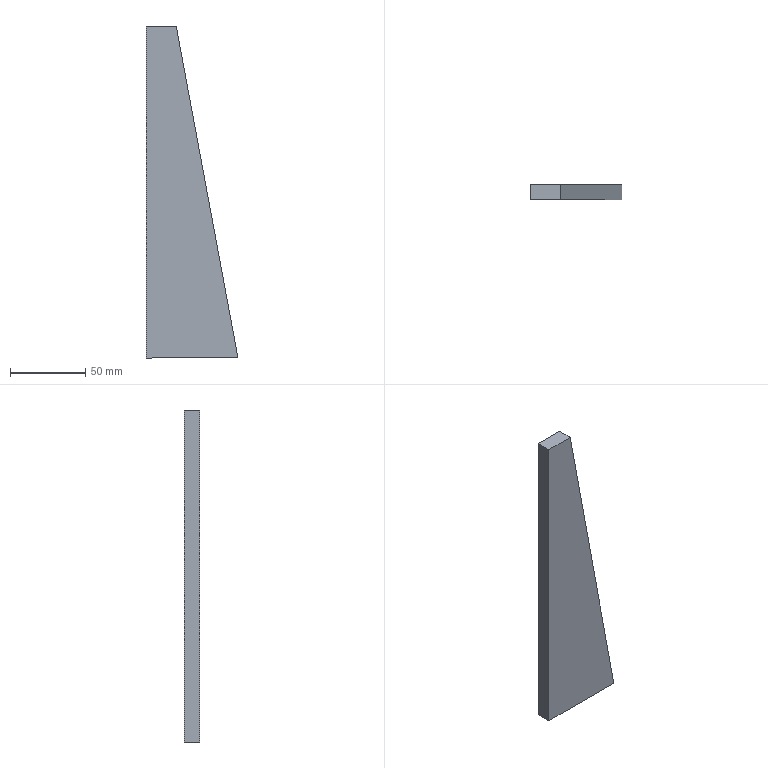Part | SolidWorks | features BaseBody 1 | 1 solid | 6 faces | box 60.857 x 10 x 220 mm | volume 88943 mm3 | plane 6
STEP:
#1=CARTESIAN_POINT('',(50.,2027.,-500.));
#2=VERTEX_POINT('',#1);
#3=CARTESIAN_POINT('',(30.,2027.,-500.));
#4=VERTEX_POINT('',#3);
#5=CARTESIAN_POINT('',(240.,2027.,-500.));
#6=DIRECTION('',(-1.,0.,0.));
#7=VECTOR('',#6,1000.);
#8=LINE('',#5,#7);
#9=EDGE_CURVE('',#2,#4,#8,.T.);
#10=ORIENTED_EDGE('',*,*,#9,.T.);
#11=CARTESIAN_POINT('',(30.,2027.,-720.));
#12=VERTEX_POINT('',#11);
#13=CARTESIAN_POINT('',(30.,2027.,-1330.));
#14=DIRECTION('',(0.,0.,-1.));
#15=VECTOR('',#14,1000.);
#16=LINE('',#13,#15);
#17=EDGE_CURVE('',#4,#12,#16,.T.);
#18=ORIENTED_EDGE('',*,*,#17,.T.);
#19=CARTESIAN_POINT('',(90.857,2027.,-720.));
#20=VERTEX_POINT('',#19);
#21=CARTESIAN_POINT('',(240.,2027.,-720.));
#22=DIRECTION('',(1.,0.,0.));
#23=VECTOR('',#22,1000.);
#24=LINE('',#21,#23);
#25=EDGE_CURVE('',#12,#20,#24,.T.);
#26=ORIENTED_EDGE('',*,*,#25,.T.);
#27=CARTESIAN_POINT('',(90.857,2027.,-720.));
#28=DIRECTION('',(-0.1826,0.,0.9832));
#29=VECTOR('',#28,1000.);
#30=LINE('',#27,#29);
#31=EDGE_CURVE('',#20,#2,#30,.T.);
#32=ORIENTED_EDGE('',*,*,#31,.T.);
#33=EDGE_LOOP('',(#10,#18,#26,#32));
#34=FACE_OUTER_BOUND('',#33,.T.);
#35=CARTESIAN_POINT('',(240.,2027.,-1330.));
#36=DIRECTION('',(0.,-1.,0.));
#37=DIRECTION('',(0.,0.,-1.));
#38=AXIS2_PLACEMENT_3D('',#35,#36,#37);
#39=PLANE('',#38);
#40=ADVANCED_FACE('',(#34),#39,.T.);
#41=CARTESIAN_POINT('',(30.,2037.,-500.));
#42=VERTEX_POINT('',#41);
#43=CARTESIAN_POINT('',(30.,2027.,-500.));
#44=DIRECTION('',(0.,1.,0.));
#45=VECTOR('',#44,1000.);
#46=LINE('',#43,#45);
#47=EDGE_CURVE('',#4,#42,#46,.T.);
#48=ORIENTED_EDGE('',*,*,#47,.T.);
#49=CARTESIAN_POINT('',(30.,2037.,-720.));
#50=VERTEX_POINT('',#49);
#51=CARTESIAN_POINT('',(30.,2037.,-1300.));
#52=DIRECTION('',(0.,0.,-1.));
#53=VECTOR('',#52,1000.);
#54=LINE('',#51,#53);
#55=EDGE_CURVE('',#42,#50,#54,.T.);
#56=ORIENTED_EDGE('',*,*,#55,.T.);
#57=CARTESIAN_POINT('',(30.,2027.,-720.));
#58=DIRECTION('',(0.,-1.,0.));
#59=VECTOR('',#58,1000.);
#60=LINE('',#57,#59);
#61=EDGE_CURVE('',#50,#12,#60,.T.);
#62=ORIENTED_EDGE('',*,*,#61,.T.);
#63=ORIENTED_EDGE('',*,*,#17,.F.);
#64=EDGE_LOOP('',(#48,#56,#62,#63));
#65=FACE_OUTER_BOUND('',#64,.T.);
#66=CARTESIAN_POINT('',(30.,2027.,-1300.));
#67=DIRECTION('',(-1.,0.,0.));
#68=DIRECTION('',(0.,0.,1.));
#69=AXIS2_PLACEMENT_3D('',#66,#67,#68);
#70=PLANE('',#69);
#71=ADVANCED_FACE('',(#65),#70,.T.);
#72=CARTESIAN_POINT('',(50.,2037.,-500.));
#73=VERTEX_POINT('',#72);
#74=CARTESIAN_POINT('',(50.,2027.,-500.));
#75=DIRECTION('',(0.,1.,0.));
#76=VECTOR('',#75,1000.);
#77=LINE('',#74,#76);
#78=EDGE_CURVE('',#2,#73,#77,.T.);
#79=ORIENTED_EDGE('',*,*,#78,.T.);
#80=CARTESIAN_POINT('',(30.,2037.,-500.));
#81=DIRECTION('',(-1.,0.,0.));
#82=VECTOR('',#81,1000.);
#83=LINE('',#80,#82);
#84=EDGE_CURVE('',#73,#42,#83,.T.);
#85=ORIENTED_EDGE('',*,*,#84,.T.);
#86=ORIENTED_EDGE('',*,*,#47,.F.);
#87=ORIENTED_EDGE('',*,*,#9,.F.);
#88=EDGE_LOOP('',(#79,#85,#86,#87));
#89=FACE_OUTER_BOUND('',#88,.T.);
#90=CARTESIAN_POINT('',(30.,2027.,-500.));
#91=DIRECTION('',(0.,0.,1.));
#92=DIRECTION('',(1.,0.,0.));
#93=AXIS2_PLACEMENT_3D('',#90,#91,#92);
#94=PLANE('',#93);
#95=ADVANCED_FACE('',(#89),#94,.T.);
#96=ORIENTED_EDGE('',*,*,#78,.F.);
#97=ORIENTED_EDGE('',*,*,#31,.F.);
#98=CARTESIAN_POINT('',(90.857,2037.,-720.));
#99=VERTEX_POINT('',#98);
#100=CARTESIAN_POINT('',(90.857,2027.,-720.));
#101=DIRECTION('',(0.,1.,0.));
#102=VECTOR('',#101,1000.);
#103=LINE('',#100,#102);
#104=EDGE_CURVE('',#20,#99,#103,.T.);
#105=ORIENTED_EDGE('',*,*,#104,.T.);
#106=CARTESIAN_POINT('',(50.,2037.,-500.));
#107=DIRECTION('',(-0.1826,0.,0.9832));
#108=VECTOR('',#107,1000.);
#109=LINE('',#106,#108);
#110=EDGE_CURVE('',#99,#73,#109,.T.);
#111=ORIENTED_EDGE('',*,*,#110,.T.);
#112=EDGE_LOOP('',(#96,#97,#105,#111));
#113=FACE_OUTER_BOUND('',#112,.T.);
#114=CARTESIAN_POINT('',(50.,2027.,-500.));
#115=DIRECTION('',(0.9832,0.,0.1826));
#116=DIRECTION('',(0.1826,0.,-0.9832));
#117=AXIS2_PLACEMENT_3D('',#114,#115,#116);
#118=PLANE('',#117);
#119=ADVANCED_FACE('',(#113),#118,.T.);
#120=ORIENTED_EDGE('',*,*,#104,.F.);
#121=ORIENTED_EDGE('',*,*,#25,.F.);
#122=ORIENTED_EDGE('',*,*,#61,.F.);
#123=CARTESIAN_POINT('',(-240.,2037.,-720.));
#124=DIRECTION('',(1.,0.,0.));
#125=VECTOR('',#124,1000.);
#126=LINE('',#123,#125);
#127=EDGE_CURVE('',#50,#99,#126,.T.);
#128=ORIENTED_EDGE('',*,*,#127,.T.);
#129=EDGE_LOOP('',(#120,#121,#122,#128));
#130=FACE_OUTER_BOUND('',#129,.T.);
#131=CARTESIAN_POINT('',(-240.,2402.,-720.));
#132=DIRECTION('',(0.,0.,-1.));
#133=DIRECTION('',(-1.,0.,0.));
#134=AXIS2_PLACEMENT_3D('',#131,#132,#133);
#135=PLANE('',#134);
#136=ADVANCED_FACE('',(#130),#135,.T.);
#137=ORIENTED_EDGE('',*,*,#84,.F.);
#138=ORIENTED_EDGE('',*,*,#110,.F.);
#139=ORIENTED_EDGE('',*,*,#127,.F.);
#140=ORIENTED_EDGE('',*,*,#55,.F.);
#141=EDGE_LOOP('',(#137,#138,#139,#140));
#142=FACE_OUTER_BOUND('',#141,.T.);
#143=CARTESIAN_POINT('',(240.,2037.,-1330.));
#144=DIRECTION('',(0.,-1.,0.));
#145=DIRECTION('',(0.,0.,-1.));
#146=AXIS2_PLACEMENT_3D('',#143,#144,#145);
#147=PLANE('',#146);
#148=ADVANCED_FACE('',(#142),#147,.F.);
#149=CLOSED_SHELL('',(#40,#71,#95,#119,#136,#148));
#150=MANIFOLD_SOLID_BREP('',#149);
#151=CARTESIAN_POINT('',(0.,0.,0.));
#152=DIRECTION('',(0.,0.,1.));
#153=DIRECTION('',(1.,0.,0.));
#154=AXIS2_PLACEMENT_3D('',#151,#152,#153);
#155=(LENGTH_UNIT()NAMED_UNIT(*)SI_UNIT(.MILLI.,.METRE.));
#156=UNCERTAINTY_MEASURE_WITH_UNIT(LENGTH_MEASURE(0.00001),#155,'','');
#157=(NAMED_UNIT(*)PLANE_ANGLE_UNIT()SI_UNIT($,.RADIAN.));
#158=(NAMED_UNIT(*)SI_UNIT($,.STERADIAN.)SOLID_ANGLE_UNIT());
#159=(GEOMETRIC_REPRESENTATION_CONTEXT(3)GLOBAL_UNCERTAINTY_ASSIGNED_CONTEXT((#156))GLOBAL_UNIT_ASSIGNED_CONTEXT((#155,#157,#158))REPRESENTATION_CONTEXT('',''));
#160=ADVANCED_BREP_SHAPE_REPRESENTATION('',(#150,#154),#159);